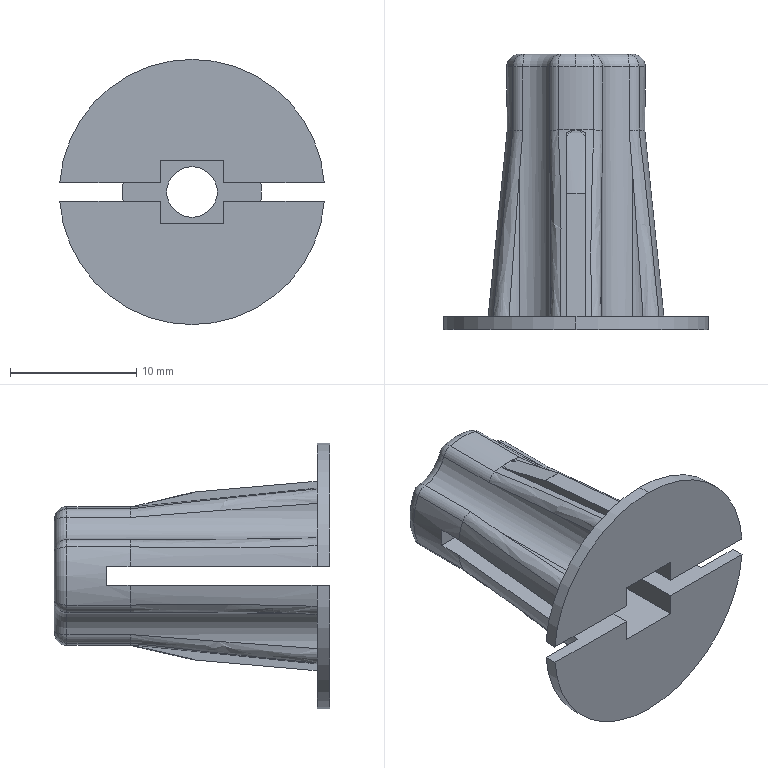Part | STEP file | PCS-P06-2_1_2.stp | 1 solid | 100 faces | box 20.946 x 21.8 x 21 mm | volume 1623 mm3 | plane 38 | cylinder 26 | cone 11 | torus 9 | spline 8 | sphere 8 | commonest cylinder face diameters 2 x8 5 x6 11 x5 4 x4 21 x3